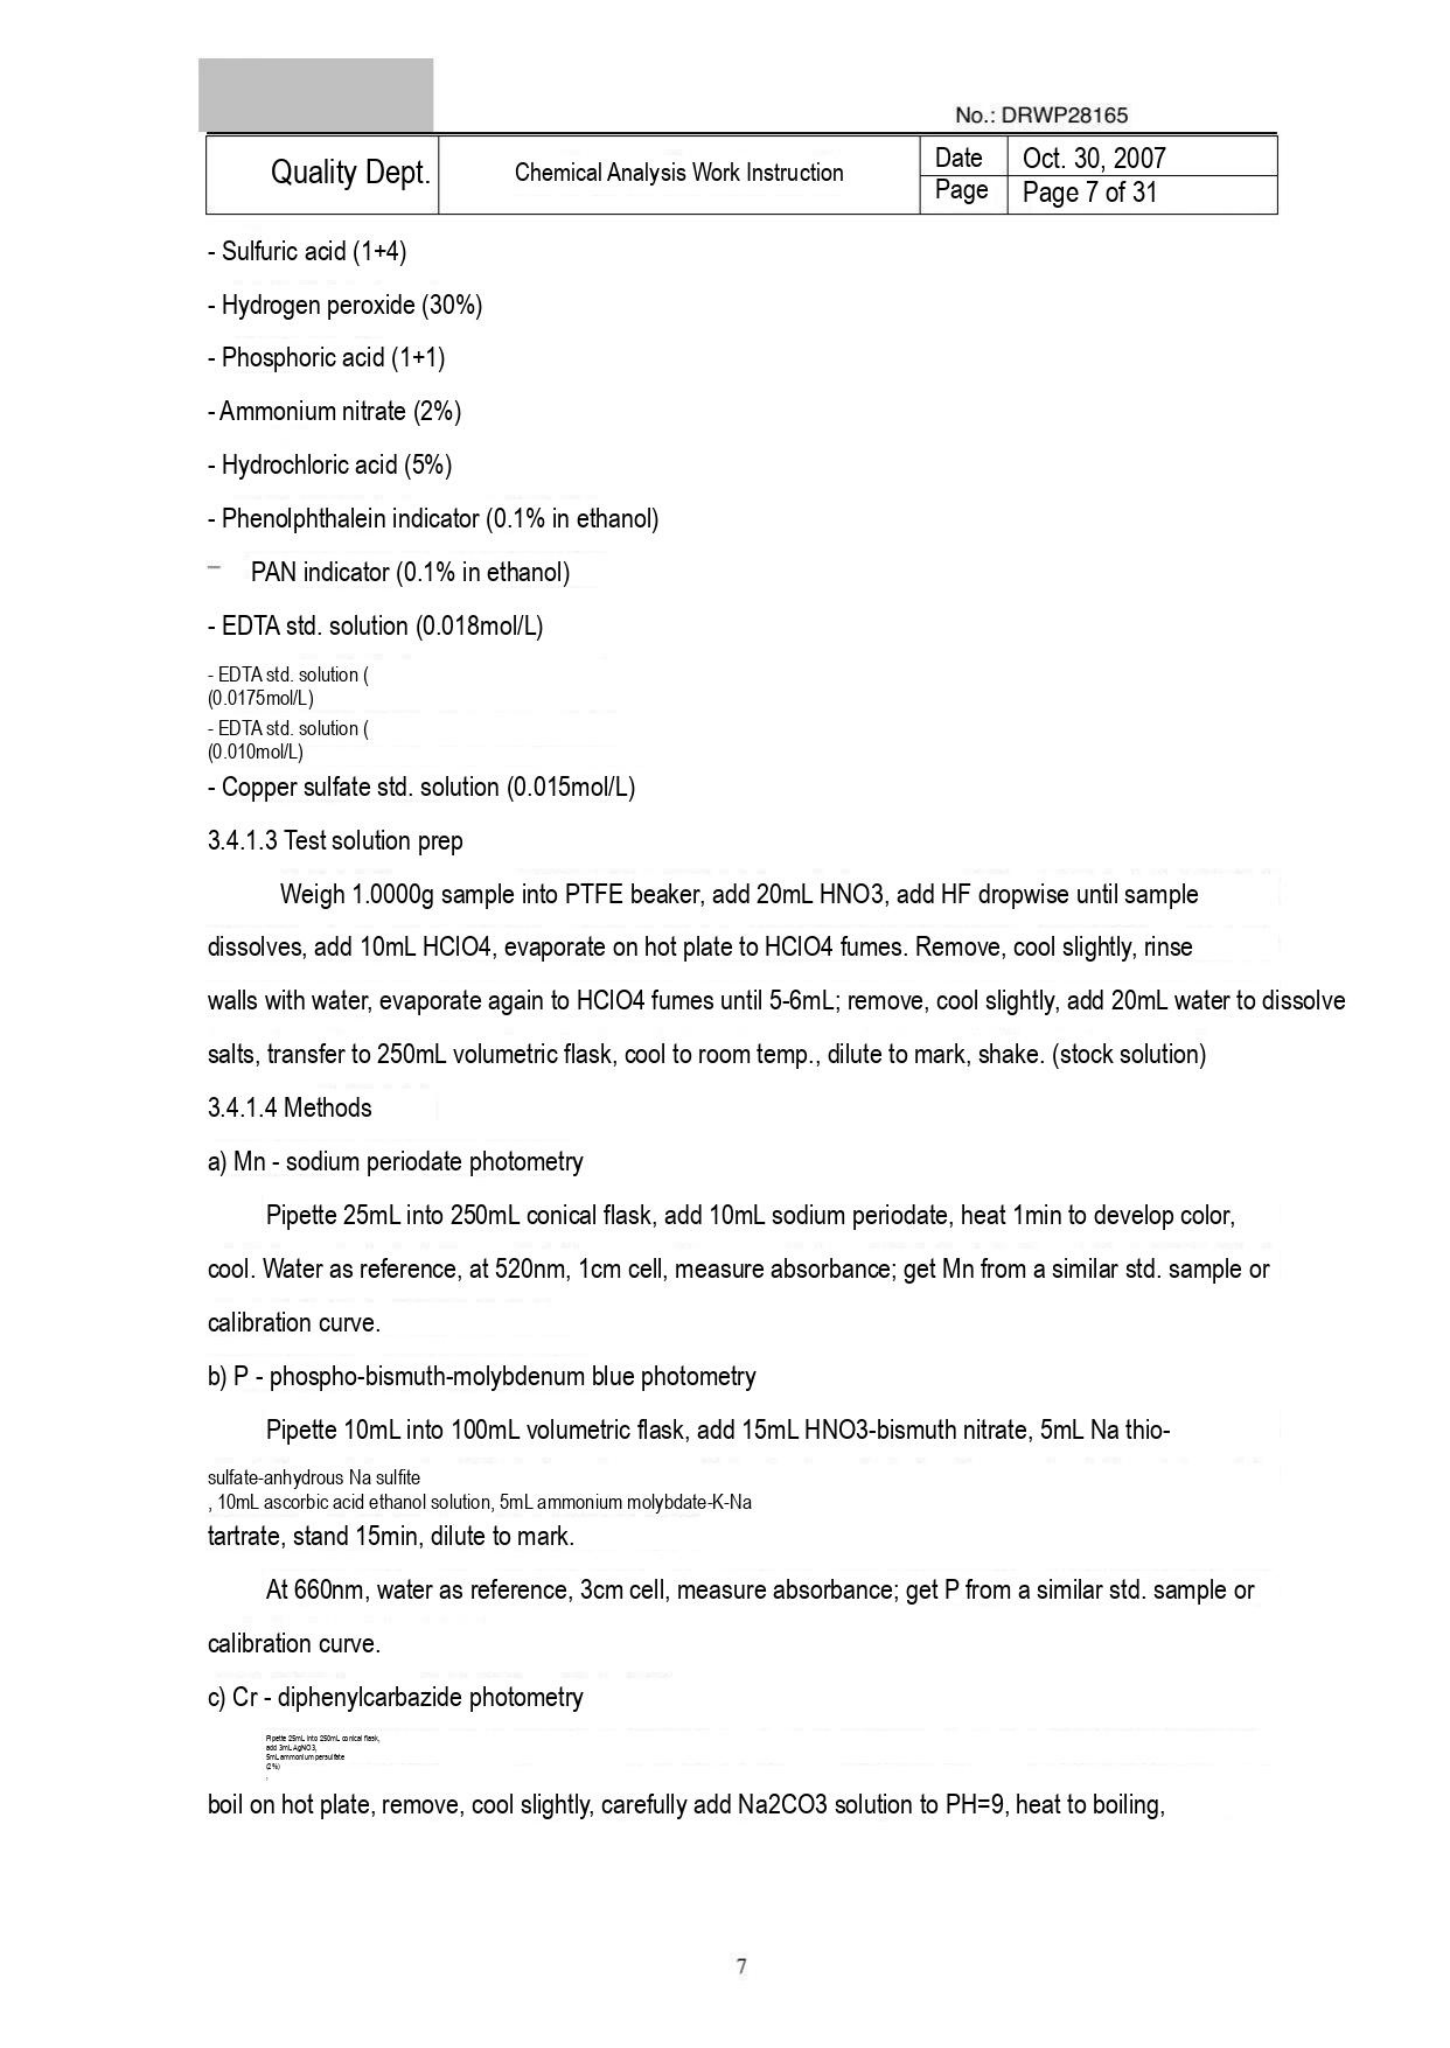No.: DRWP28165

| Quality Dept. | Chemical Analysis Work Instruction | Date | Oct. 30, 2007 |
|---|---|---|---|
| | | Page | Page 7 of 31 |

- Sulfuric acid (1+4)

- Hydrogen peroxide (30%)

- Phosphoric acid (1+1)

- Ammonium nitrate (2%)

- Hydrochloric acid (5%)

- Phenolphthalein indicator (0.1% in ethanol)

– PAN indicator (0.1% in ethanol)

- EDTA std. solution (0.018mol/L)

- EDTA std. solution (
(0.0175mol/L)

- EDTA std. solution (
(0.010mol/L)

- Copper sulfate std. solution (0.015mol/L)

3.4.1.3 Test solution prep

Weigh 1.0000g sample into PTFE beaker, add 20mL HNO3, add HF dropwise until sample dissolves, add 10mL HClO4, evaporate on hot plate to HClO4 fumes. Remove, cool slightly, rinse walls with water, evaporate again to HClO4 fumes until 5-6mL; remove, cool slightly, add 20mL water to dissolve salts, transfer to 250mL volumetric flask, cool to room temp., dilute to mark, shake. (stock solution)

3.4.1.4 Methods

a) Mn - sodium periodate photometry

Pipette 25mL into 250mL conical flask, add 10mL sodium periodate, heat 1min to develop color, cool. Water as reference, at 520nm, 1cm cell, measure absorbance; get Mn from a similar std. sample or calibration curve.

b) P - phospho-bismuth-molybdenum blue photometry

Pipette 10mL into 100mL volumetric flask, add 15mL HNO3-bismuth nitrate, 5mL Na thio-
sulfate-anhydrous Na sulfite
, 10mL ascorbic acid ethanol solution, 5mL ammonium molybdate-K-Na
tartrate, stand 15min, dilute to mark.

At 660nm, water as reference, 3cm cell, measure absorbance; get P from a similar std. sample or calibration curve.

c) Cr - diphenylcarbazide photometry

Pipette 25mL into 250mL conical flask,
add 3mL AgNO3,
5mL ammonium persulfate
(2%)

boil on hot plate, remove, cool slightly, carefully add Na2CO3 solution to PH=9, heat to boiling,

7
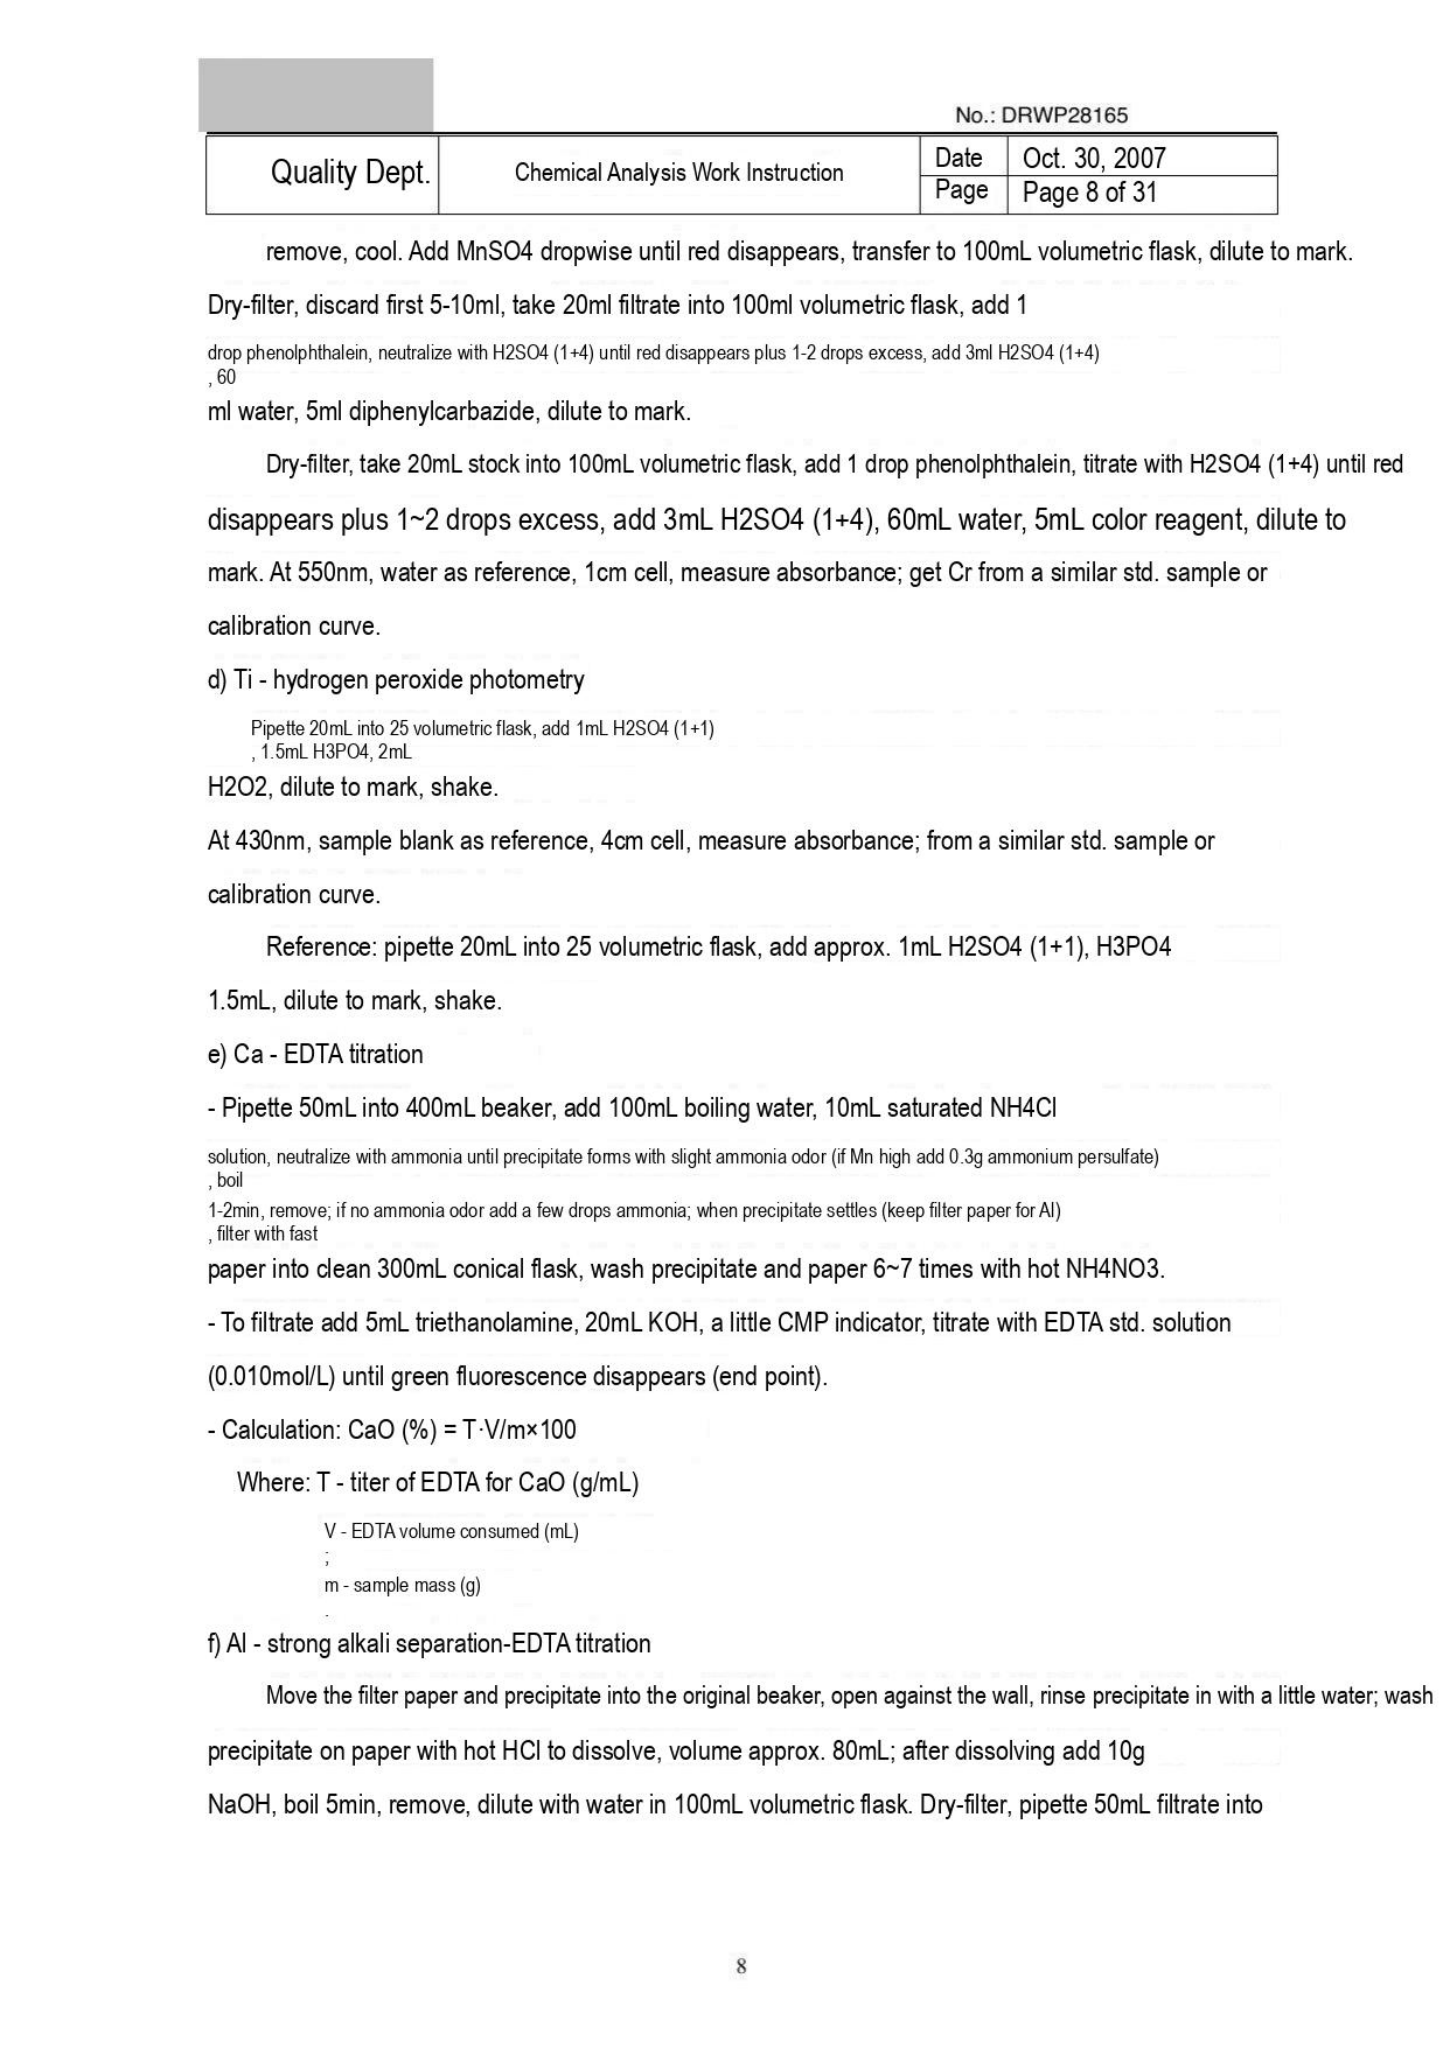No.: DRWP28165

| Quality Dept. | Chemical Analysis Work Instruction | Date | Oct. 30, 2007 |
|---|---|---|---|
| | | Page | Page 8 of 31 |

remove, cool. Add MnSO4 dropwise until red disappears, transfer to 100mL volumetric flask, dilute to mark.

Dry-filter, discard first 5-10ml, take 20ml filtrate into 100ml volumetric flask, add 1

drop phenolphthalein, neutralize with H2SO4 (1+4) until red disappears plus 1-2 drops excess, add 3ml H2SO4 (1+4)
, 60
ml water, 5ml diphenylcarbazide, dilute to mark.

Dry-filter, take 20mL stock into 100mL volumetric flask, add 1 drop phenolphthalein, titrate with H2SO4 (1+4) until red disappears plus 1~2 drops excess, add 3mL H2SO4 (1+4), 60mL water, 5mL color reagent, dilute to mark. At 550nm, water as reference, 1cm cell, measure absorbance; get Cr from a similar std. sample or calibration curve.

d) Ti - hydrogen peroxide photometry

Pipette 20mL into 25 volumetric flask, add 1mL H2SO4 (1+1)
, 1.5mL H3PO4, 2mL
H2O2, dilute to mark, shake.

At 430nm, sample blank as reference, 4cm cell, measure absorbance; from a similar std. sample or calibration curve.

Reference: pipette 20mL into 25 volumetric flask, add approx. 1mL H2SO4 (1+1), H3PO4 1.5mL, dilute to mark, shake.

e) Ca - EDTA titration

- Pipette 50mL into 400mL beaker, add 100mL boiling water, 10mL saturated NH4Cl

solution, neutralize with ammonia until precipitate forms with slight ammonia odor (if Mn high add 0.3g ammonium persulfate)
, boil
1-2min, remove; if no ammonia odor add a few drops ammonia; when precipitate settles (keep filter paper for Al)
, filter with fast
paper into clean 300mL conical flask, wash precipitate and paper 6~7 times with hot NH4NO3.

- To filtrate add 5mL triethanolamine, 20mL KOH, a little CMP indicator, titrate with EDTA std. solution (0.010mol/L) until green fluorescence disappears (end point).

- Calculation: CaO (%) = T·V/m×100

Where: T - titer of EDTA for CaO (g/mL)

V - EDTA volume consumed (mL)
;
m - sample mass (g)
.

f) Al - strong alkali separation-EDTA titration

Move the filter paper and precipitate into the original beaker, open against the wall, rinse precipitate in with a little water; wash precipitate on paper with hot HCl to dissolve, volume approx. 80mL; after dissolving add 10g NaOH, boil 5min, remove, dilute with water in 100mL volumetric flask. Dry-filter, pipette 50mL filtrate into

8
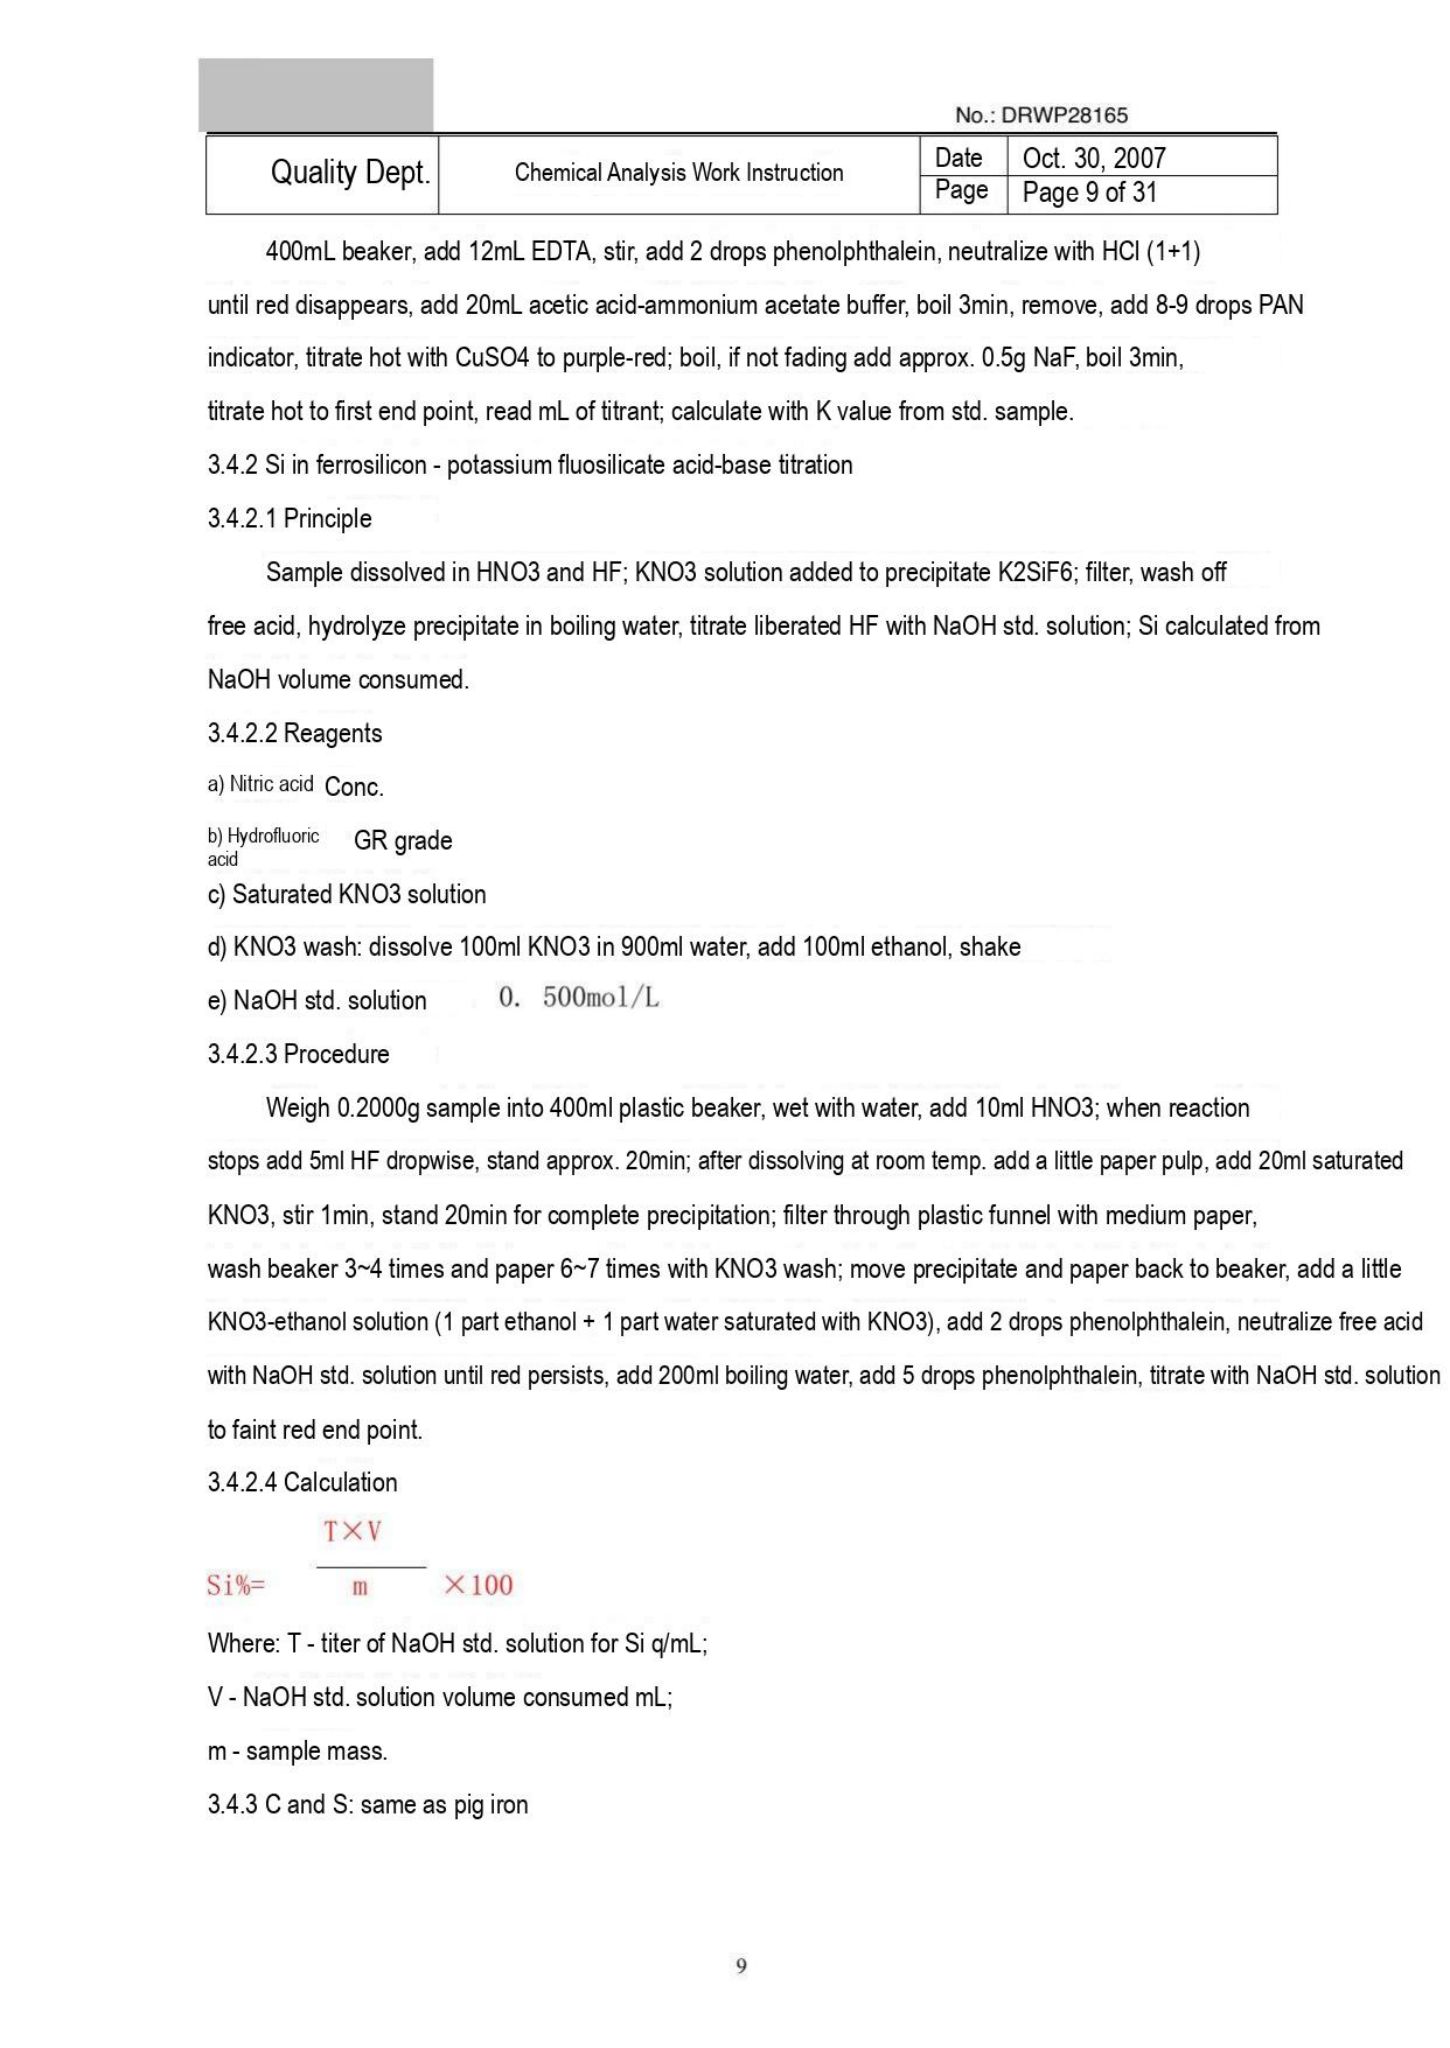No.: DRWP28165

| Quality Dept. | Chemical Analysis Work Instruction | Date | Oct. 30, 2007 |
|---|---|---|---|
| | | Page | Page 9 of 31 |

400mL beaker, add 12mL EDTA, stir, add 2 drops phenolphthalein, neutralize with HCl (1+1) until red disappears, add 20mL acetic acid-ammonium acetate buffer, boil 3min, remove, add 8-9 drops PAN indicator, titrate hot with CuSO4 to purple-red; boil, if not fading add approx. 0.5g NaF, boil 3min, titrate hot to first end point, read mL of titrant; calculate with K value from std. sample.

3.4.2 Si in ferrosilicon - potassium fluosilicate acid-base titration

3.4.2.1 Principle

Sample dissolved in HNO3 and HF; KNO3 solution added to precipitate K2SiF6; filter, wash off free acid, hydrolyze precipitate in boiling water, titrate liberated HF with NaOH std. solution; Si calculated from NaOH volume consumed.

3.4.2.2 Reagents

a) Nitric acid Conc.

b) Hydrofluoric acid GR grade

c) Saturated KNO3 solution

d) KNO3 wash: dissolve 100ml KNO3 in 900ml water, add 100ml ethanol, shake

e) NaOH std. solution 0. 500mol/L

3.4.2.3 Procedure

Weigh 0.2000g sample into 400ml plastic beaker, wet with water, add 10ml HNO3; when reaction stops add 5ml HF dropwise, stand approx. 20min; after dissolving at room temp. add a little paper pulp, add 20ml saturated KNO3, stir 1min, stand 20min for complete precipitation; filter through plastic funnel with medium paper, wash beaker 3~4 times and paper 6~7 times with KNO3 wash; move precipitate and paper back to beaker, add a little KNO3-ethanol solution (1 part ethanol + 1 part water saturated with KNO3), add 2 drops phenolphthalein, neutralize free acid with NaOH std. solution until red persists, add 200ml boiling water, add 5 drops phenolphthalein, titrate with NaOH std. solution to faint red end point.

3.4.2.4 Calculation

Si%= (T×V / m) ×100

Where: T - titer of NaOH std. solution for Si g/mL;

V - NaOH std. solution volume consumed mL;

m - sample mass.

3.4.3 C and S: same as pig iron

9
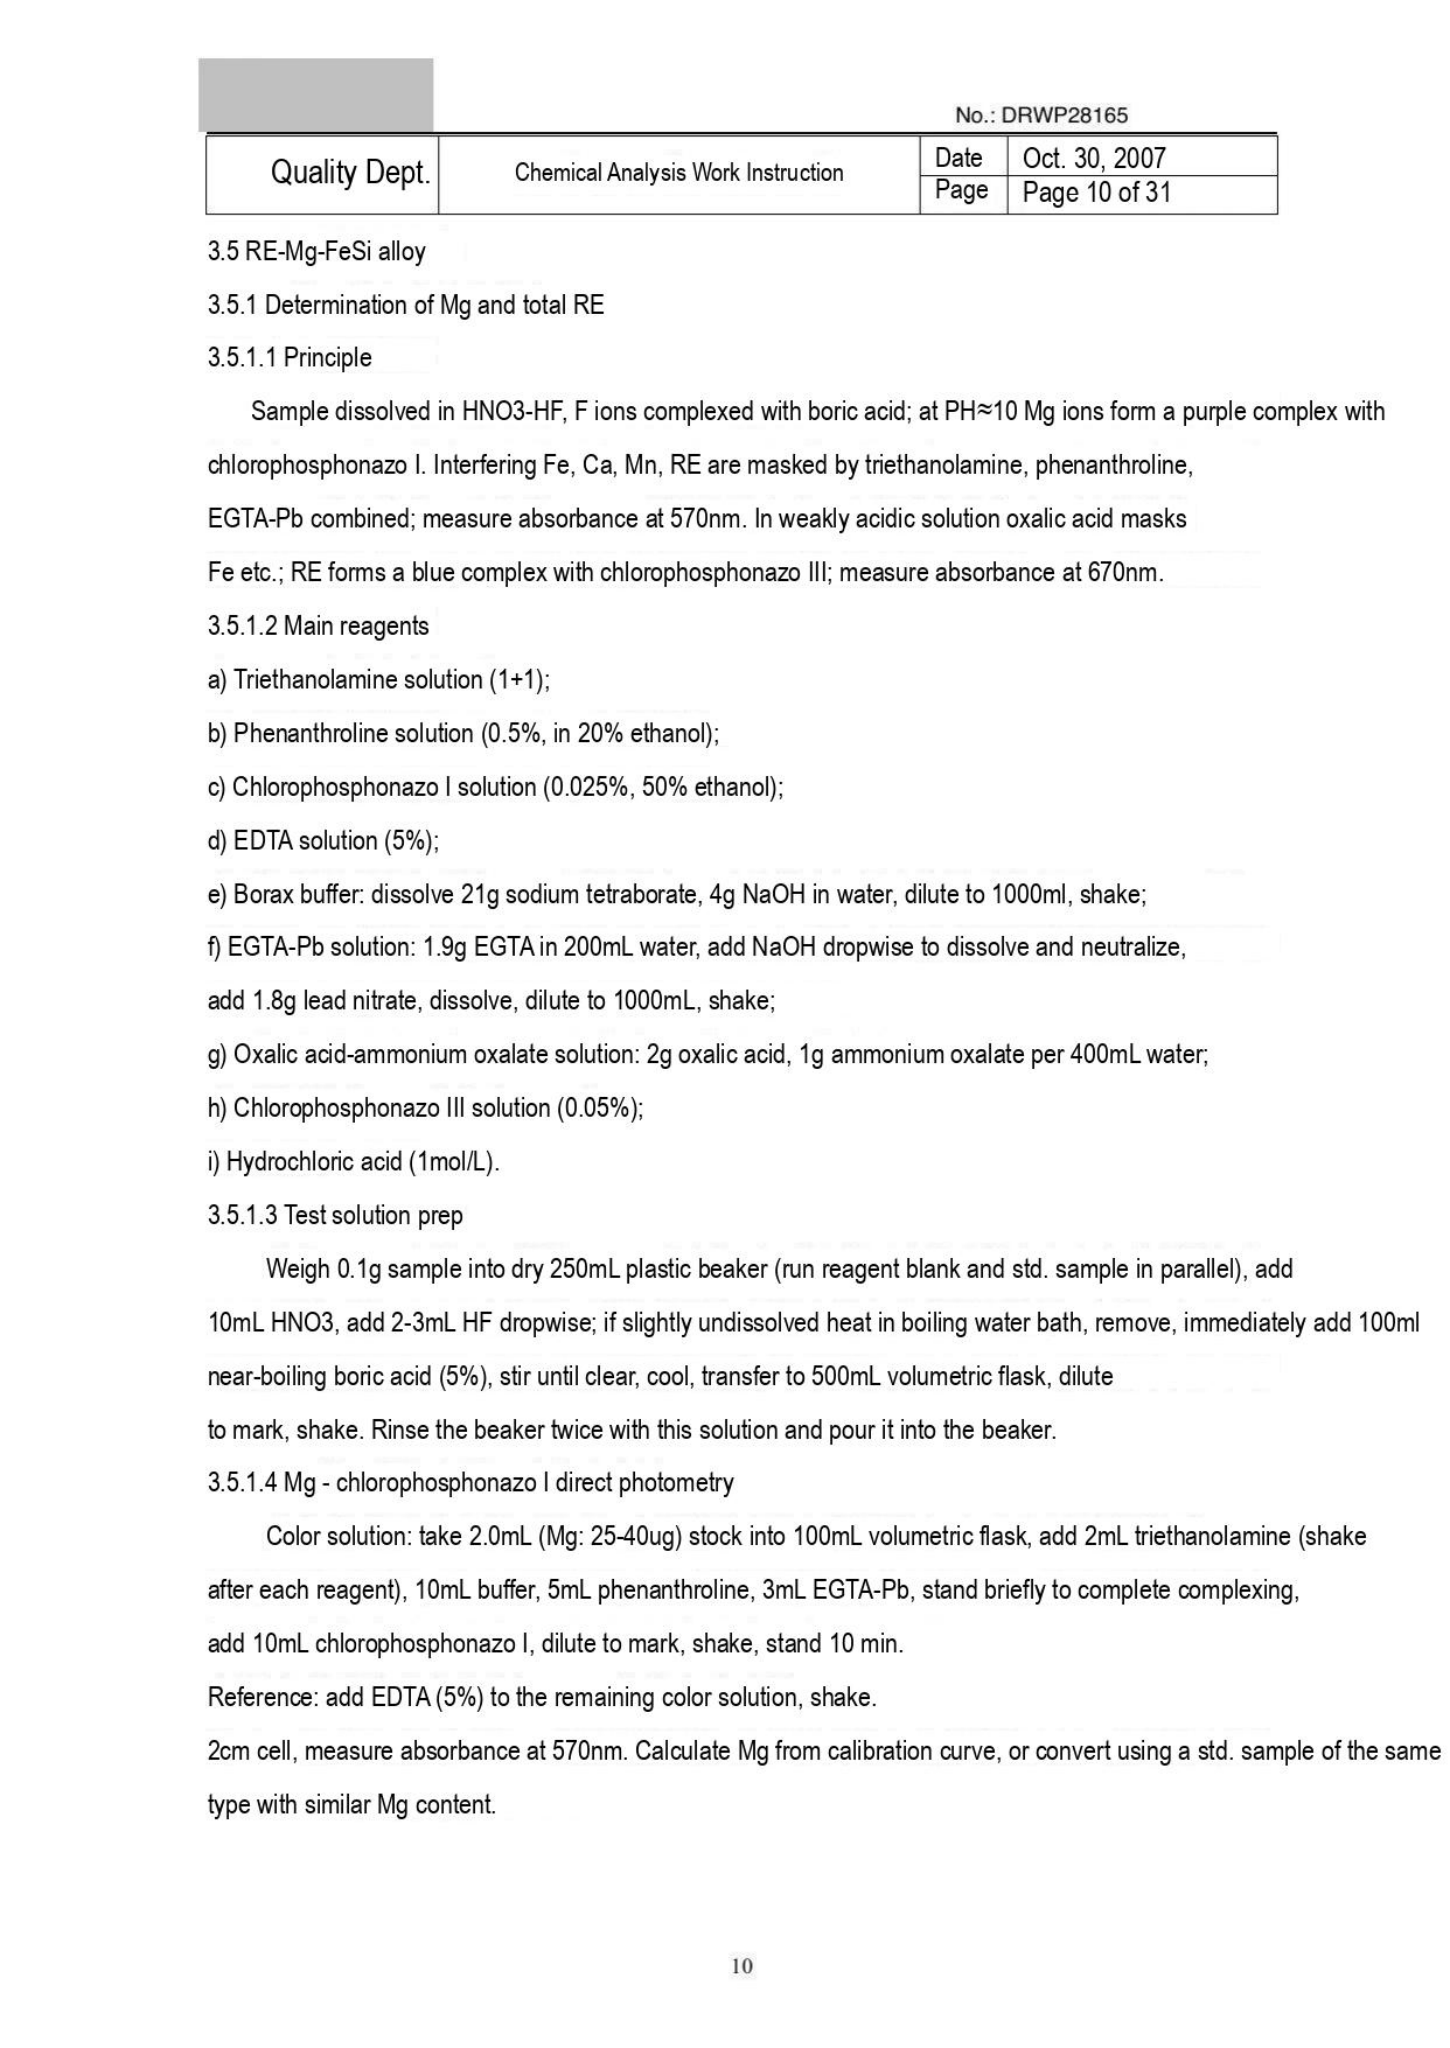No.: DRWP28165

| Quality Dept. | Chemical Analysis Work Instruction | Date | Oct. 30, 2007 |
|---|---|---|---|
| | | Page | Page 10 of 31 |

3.5 RE-Mg-FeSi alloy

3.5.1 Determination of Mg and total RE

3.5.1.1 Principle

Sample dissolved in HNO3-HF, F ions complexed with boric acid; at PH≈10 Mg ions form a purple complex with chlorophosphonazo I. Interfering Fe, Ca, Mn, RE are masked by triethanolamine, phenanthroline, EGTA-Pb combined; measure absorbance at 570nm. In weakly acidic solution oxalic acid masks Fe etc.; RE forms a blue complex with chlorophosphonazo III; measure absorbance at 670nm.

3.5.1.2 Main reagents

a) Triethanolamine solution (1+1);

b) Phenanthroline solution (0.5%, in 20% ethanol);

c) Chlorophosphonazo I solution (0.025%, 50% ethanol);

d) EDTA solution (5%);

e) Borax buffer: dissolve 21g sodium tetraborate, 4g NaOH in water, dilute to 1000ml, shake;

f) EGTA-Pb solution: 1.9g EGTA in 200mL water, add NaOH dropwise to dissolve and neutralize, add 1.8g lead nitrate, dissolve, dilute to 1000mL, shake;

g) Oxalic acid-ammonium oxalate solution: 2g oxalic acid, 1g ammonium oxalate per 400mL water;

h) Chlorophosphonazo III solution (0.05%);

i) Hydrochloric acid (1mol/L).

3.5.1.3 Test solution prep

Weigh 0.1g sample into dry 250mL plastic beaker (run reagent blank and std. sample in parallel), add 10mL HNO3, add 2-3mL HF dropwise; if slightly undissolved heat in boiling water bath, remove, immediately add 100ml near-boiling boric acid (5%), stir until clear, cool, transfer to 500mL volumetric flask, dilute to mark, shake. Rinse the beaker twice with this solution and pour it into the beaker.

3.5.1.4 Mg - chlorophosphonazo I direct photometry

Color solution: take 2.0mL (Mg: 25-40ug) stock into 100mL volumetric flask, add 2mL triethanolamine (shake after each reagent), 10mL buffer, 5mL phenanthroline, 3mL EGTA-Pb, stand briefly to complete complexing, add 10mL chlorophosphonazo I, dilute to mark, shake, stand 10 min.

Reference: add EDTA (5%) to the remaining color solution, shake.

2cm cell, measure absorbance at 570nm. Calculate Mg from calibration curve, or convert using a std. sample of the same type with similar Mg content.

10
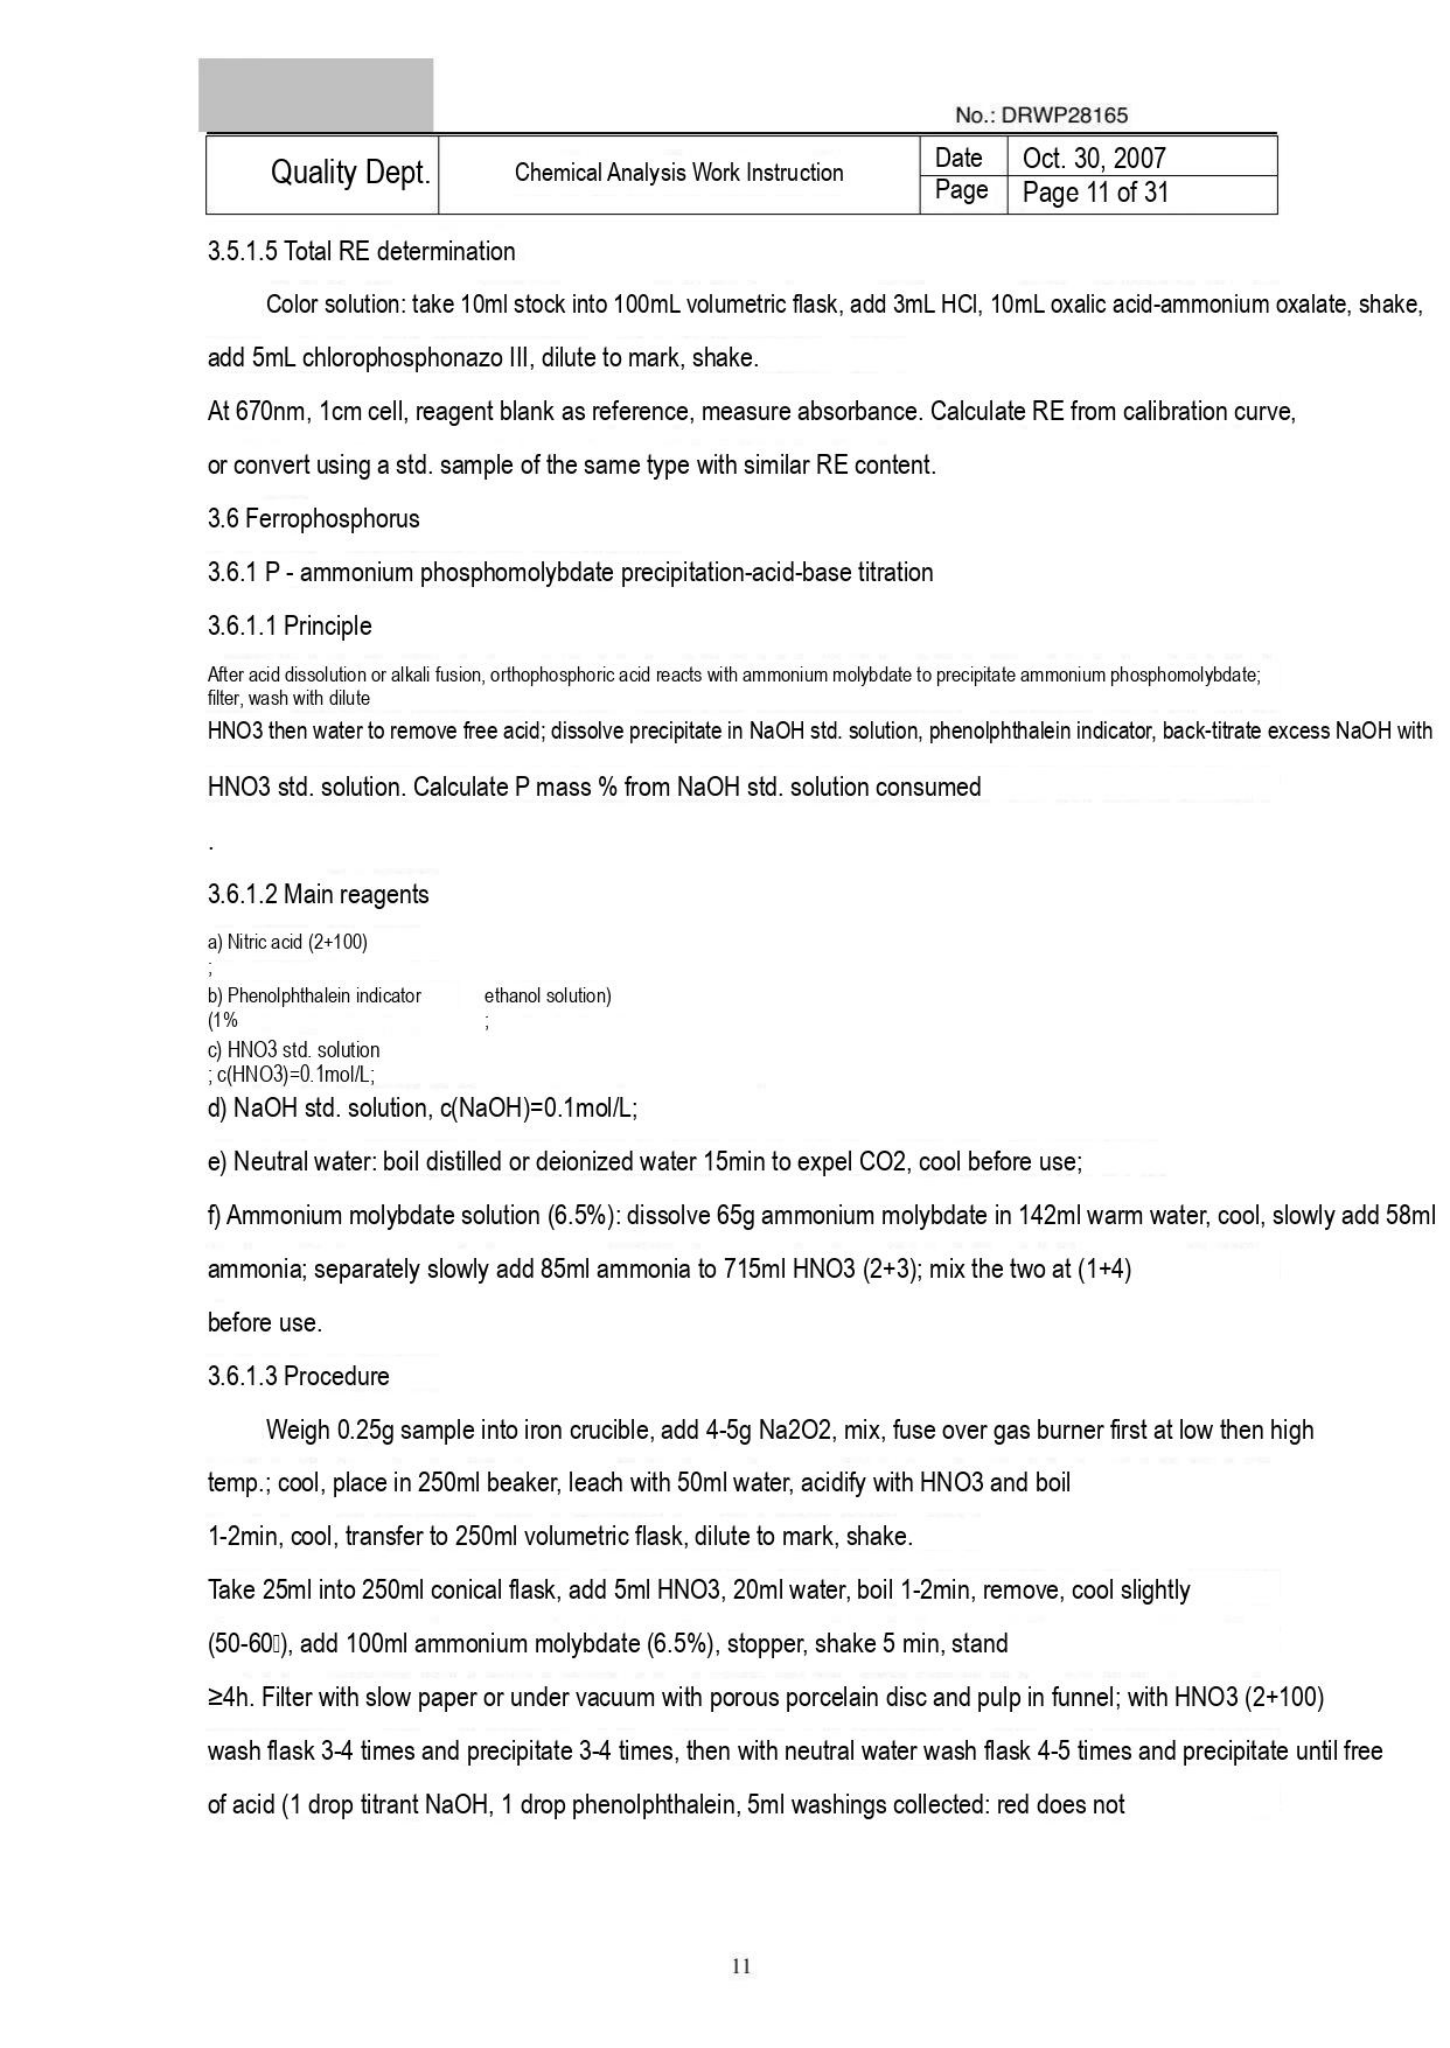No.: DRWP28165

| Quality Dept. | Chemical Analysis Work Instruction | Date | Oct. 30, 2007 |
|---|---|---|---|
| | | Page | Page 11 of 31 |

3.5.1.5 Total RE determination

Color solution: take 10ml stock into 100mL volumetric flask, add 3mL HCl, 10mL oxalic acid-ammonium oxalate, shake, add 5mL chlorophosphonazo III, dilute to mark, shake.

At 670nm, 1cm cell, reagent blank as reference, measure absorbance. Calculate RE from calibration curve, or convert using a std. sample of the same type with similar RE content.

3.6 Ferrophosphorus

3.6.1 P - ammonium phosphomolybdate precipitation-acid-base titration

3.6.1.1 Principle

After acid dissolution or alkali fusion, orthophosphoric acid reacts with ammonium molybdate to precipitate ammonium phosphomolybdate; filter, wash with dilute HNO3 then water to remove free acid; dissolve precipitate in NaOH std. solution, phenolphthalein indicator, back-titrate excess NaOH with HNO3 std. solution. Calculate P mass % from NaOH std. solution consumed

.

3.6.1.2 Main reagents

a) Nitric acid (2+100)
;
b) Phenolphthalein indicator (1% ethanol solution)
;
c) HNO3 std. solution
; c(HNO3)=0.1mol/L;
d) NaOH std. solution, c(NaOH)=0.1mol/L;

e) Neutral water: boil distilled or deionized water 15min to expel CO2, cool before use;

f) Ammonium molybdate solution (6.5%): dissolve 65g ammonium molybdate in 142ml warm water, cool, slowly add 58ml ammonia; separately slowly add 85ml ammonia to 715ml HNO3 (2+3); mix the two at (1+4) before use.

3.6.1.3 Procedure

Weigh 0.25g sample into iron crucible, add 4-5g Na2O2, mix, fuse over gas burner first at low then high temp.; cool, place in 250ml beaker, leach with 50ml water, acidify with HNO3 and boil 1-2min, cool, transfer to 250ml volumetric flask, dilute to mark, shake.

Take 25ml into 250ml conical flask, add 5ml HNO3, 20ml water, boil 1-2min, remove, cool slightly (50-60), add 100ml ammonium molybdate (6.5%), stopper, shake 5 min, stand ≥4h. Filter with slow paper or under vacuum with porous porcelain disc and pulp in funnel; with HNO3 (2+100) wash flask 3-4 times and precipitate 3-4 times, then with neutral water wash flask 4-5 times and precipitate until free of acid (1 drop titrant NaOH, 1 drop phenolphthalein, 5ml washings collected: red does not

11
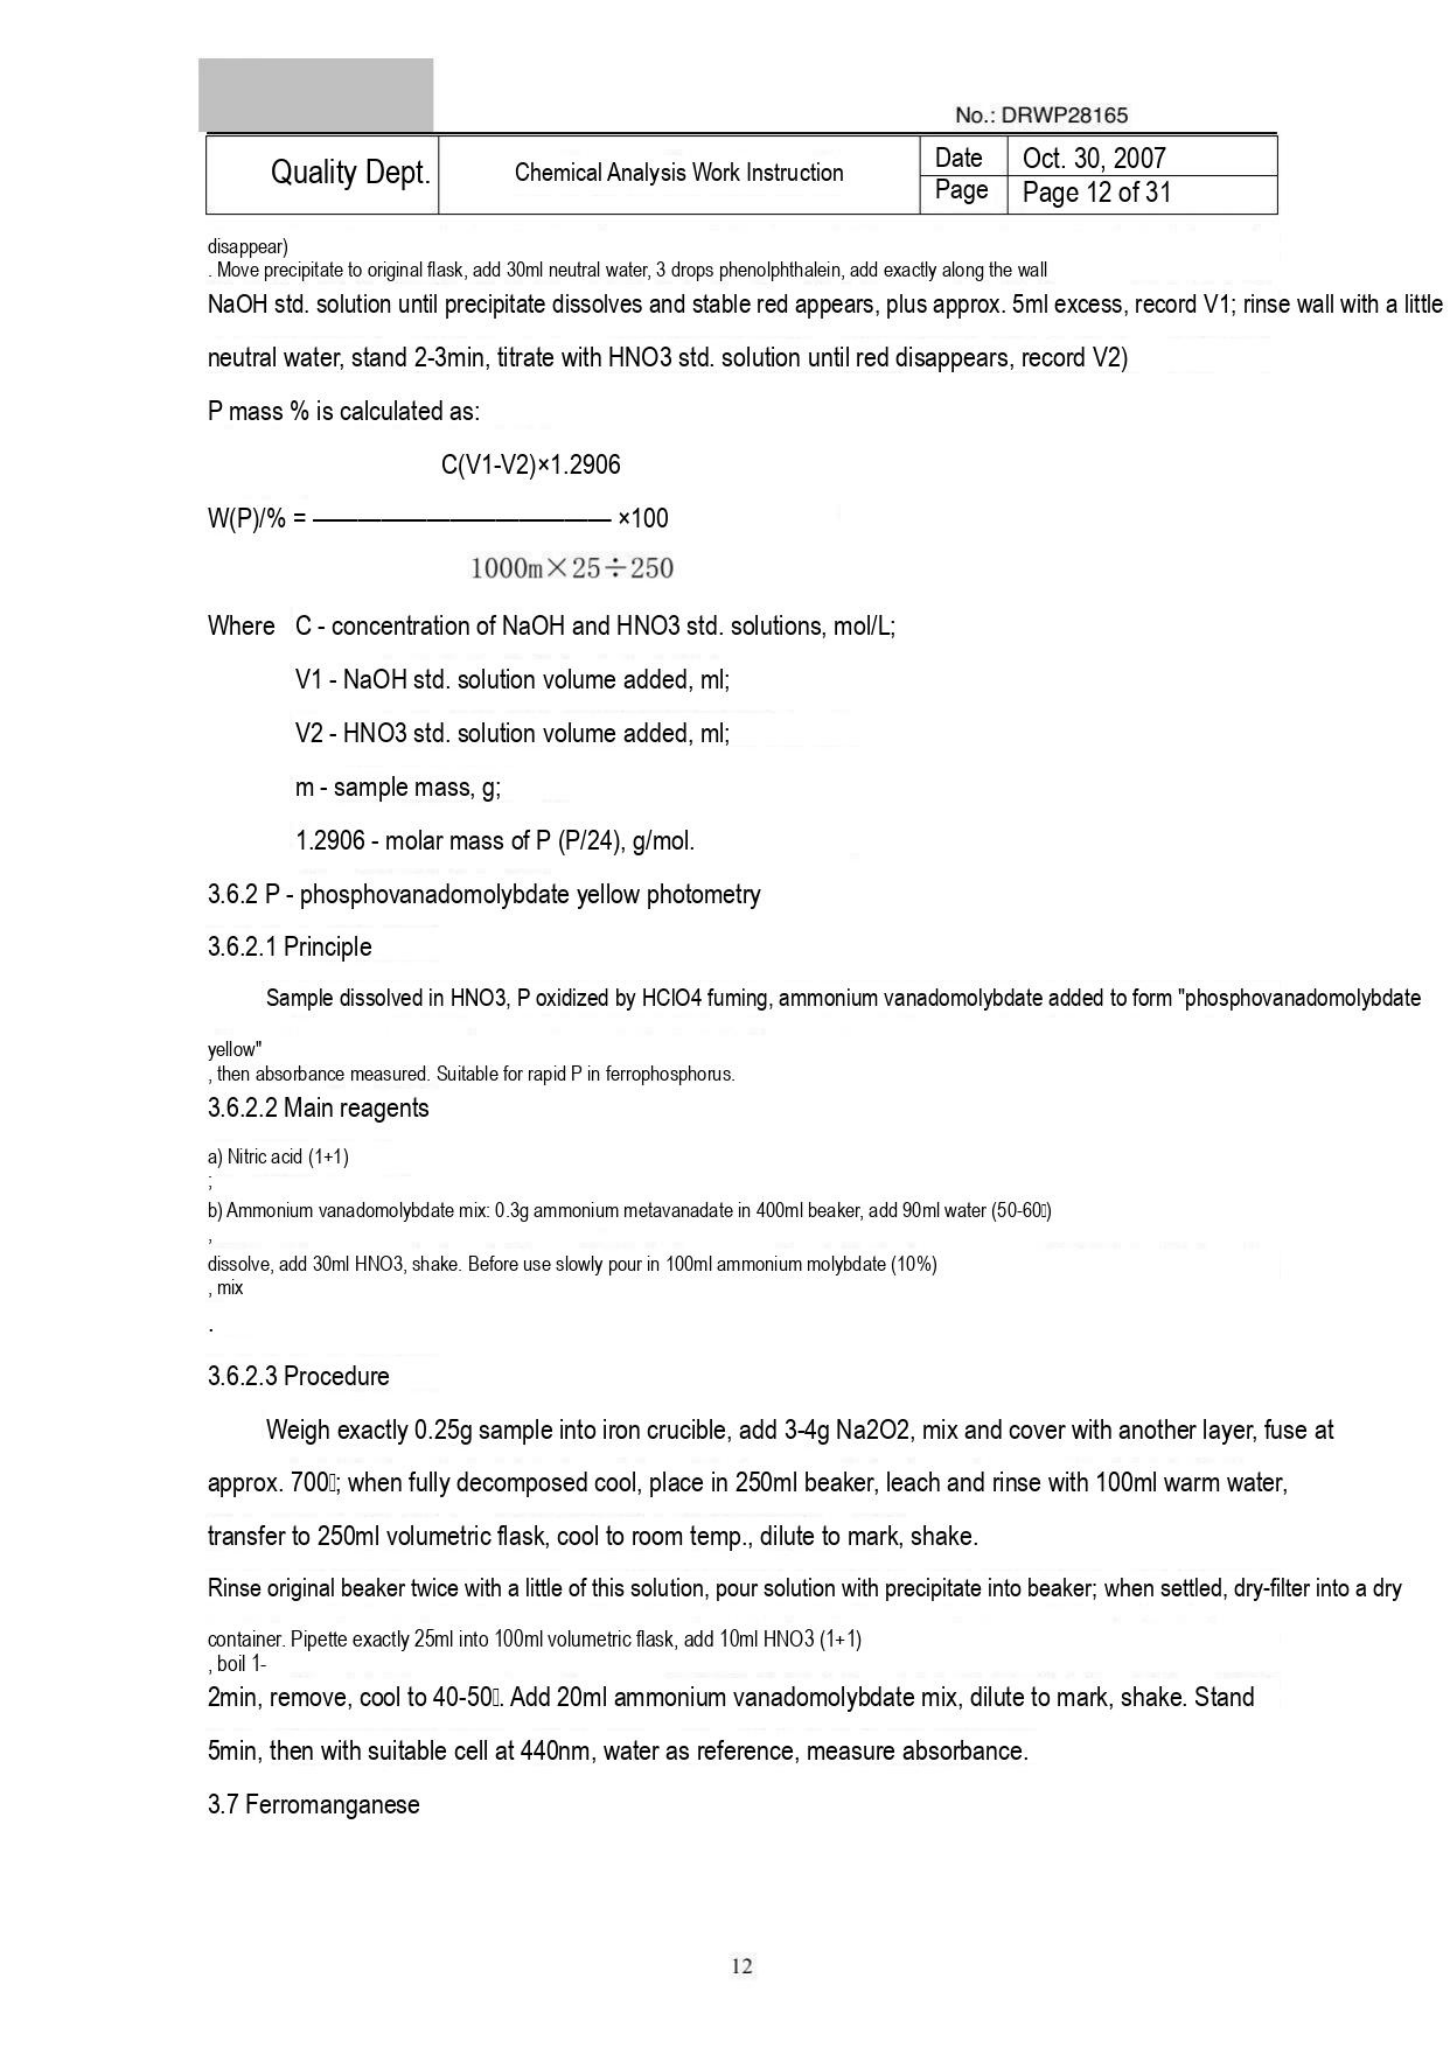No.: DRWP28165

| Quality Dept. | Chemical Analysis Work Instruction | Date | Oct. 30, 2007 |
|---|---|---|---|
| | | Page | Page 12 of 31 |

disappear)
. Move precipitate to original flask, add 30ml neutral water, 3 drops phenolphthalein, add exactly along the wall
NaOH std. solution until precipitate dissolves and stable red appears, plus approx. 5ml excess, record V1; rinse wall with a little
neutral water, stand 2-3min, titrate with HNO3 std. solution until red disappears, record V2)

P mass % is calculated as:

C(V1-V2)×1.2906
W(P)/% = ———————————— ×100
1000m×25÷250

Where C - concentration of NaOH and HNO3 std. solutions, mol/L;

V1 - NaOH std. solution volume added, ml;

V2 - HNO3 std. solution volume added, ml;

m - sample mass, g;

1.2906 - molar mass of P (P/24), g/mol.

3.6.2 P - phosphovanadomolybdate yellow photometry

3.6.2.1 Principle

Sample dissolved in HNO3, P oxidized by HClO4 fuming, ammonium vanadomolybdate added to form "phosphovanadomolybdate
yellow"
, then absorbance measured. Suitable for rapid P in ferrophosphorus.

3.6.2.2 Main reagents

a) Nitric acid (1+1)
;
b) Ammonium vanadomolybdate mix: 0.3g ammonium metavanadate in 400ml beaker, add 90ml water (50-60)
,
dissolve, add 30ml HNO3, shake. Before use slowly pour in 100ml ammonium molybdate (10%)
, mix
.

3.6.2.3 Procedure

Weigh exactly 0.25g sample into iron crucible, add 3-4g Na2O2, mix and cover with another layer, fuse at approx. 700; when fully decomposed cool, place in 250ml beaker, leach and rinse with 100ml warm water, transfer to 250ml volumetric flask, cool to room temp., dilute to mark, shake.
Rinse original beaker twice with a little of this solution, pour solution with precipitate into beaker; when settled, dry-filter into a dry
container. Pipette exactly 25ml into 100ml volumetric flask, add 10ml HNO3 (1+1)
, boil 1-
2min, remove, cool to 40-50. Add 20ml ammonium vanadomolybdate mix, dilute to mark, shake. Stand 5min, then with suitable cell at 440nm, water as reference, measure absorbance.

3.7 Ferromanganese

12